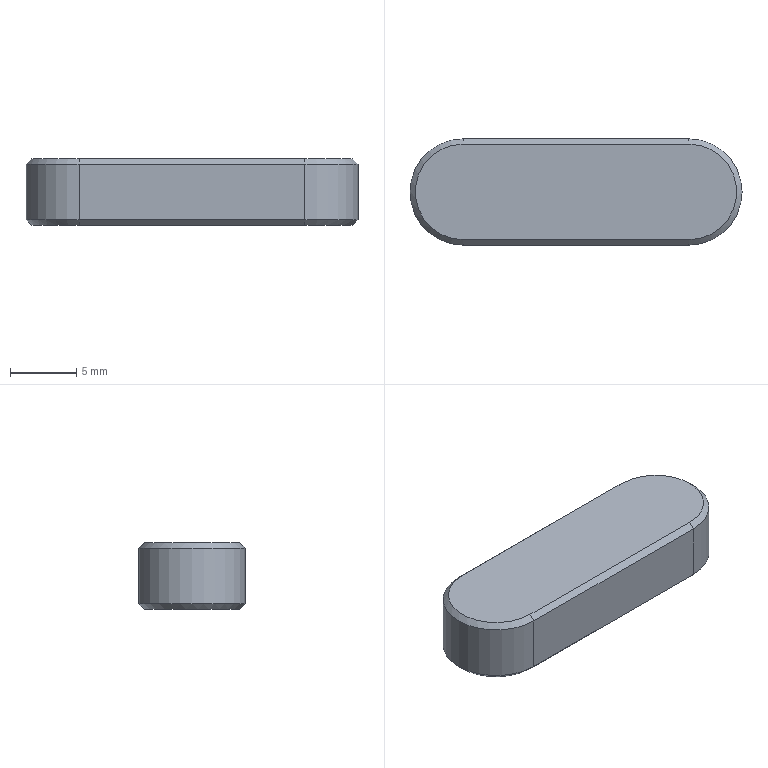Part | SolidWorks | features BaseBody 1 | 1 solid | 14 faces | box 25 x 8 x 5 mm | volume 922 mm3 | plane 8 | cone 4 | cylinder 2 | commonest cylinder face diameters 8 x2
STEP:
#1=CARTESIAN_POINT('',(21.,-3.6,-3.));
#2=VERTEX_POINT('',#1);
#3=CARTESIAN_POINT('',(21.,-4.,-2.6));
#4=VERTEX_POINT('',#3);
#5=CARTESIAN_POINT('',(21.,-3.6,-3.));
#6=DIRECTION('',(0.,-0.7071,0.7071));
#7=VECTOR('',#6,1000.);
#8=LINE('',#5,#7);
#9=EDGE_CURVE('',#2,#4,#8,.T.);
#10=ORIENTED_EDGE('',*,*,#9,.T.);
#11=CARTESIAN_POINT('',(4.,-4.,-2.6));
#12=VERTEX_POINT('',#11);
#13=CARTESIAN_POINT('',(8.25,-4.,-2.6));
#14=DIRECTION('',(-1.,0.,0.));
#15=VECTOR('',#14,1000.);
#16=LINE('',#13,#15);
#17=EDGE_CURVE('',#4,#12,#16,.T.);
#18=ORIENTED_EDGE('',*,*,#17,.T.);
#19=CARTESIAN_POINT('',(4.,-3.6,-3.));
#20=VERTEX_POINT('',#19);
#21=CARTESIAN_POINT('',(4.,-4.,-2.6));
#22=DIRECTION('',(0.,0.7071,-0.7071));
#23=VECTOR('',#22,1000.);
#24=LINE('',#21,#23);
#25=EDGE_CURVE('',#12,#20,#24,.T.);
#26=ORIENTED_EDGE('',*,*,#25,.T.);
#27=CARTESIAN_POINT('',(8.25,-3.6,-3.));
#28=DIRECTION('',(1.,0.,0.));
#29=VECTOR('',#28,1000.);
#30=LINE('',#27,#29);
#31=EDGE_CURVE('',#20,#2,#30,.T.);
#32=ORIENTED_EDGE('',*,*,#31,.T.);
#33=EDGE_LOOP('',(#10,#18,#26,#32));
#34=FACE_OUTER_BOUND('',#33,.T.);
#35=CARTESIAN_POINT('',(8.25,-3.8,-2.8));
#36=DIRECTION('',(0.,-0.7071,-0.7071));
#37=DIRECTION('',(0.,0.7071,-0.7071));
#38=AXIS2_PLACEMENT_3D('',#35,#36,#37);
#39=PLANE('',#38);
#40=ADVANCED_FACE('',(#34),#39,.T.);
#41=CARTESIAN_POINT('',(21.,3.6,-3.));
#42=VERTEX_POINT('',#41);
#43=CARTESIAN_POINT('',(21.,4.,-2.6));
#44=VERTEX_POINT('',#43);
#45=CARTESIAN_POINT('',(21.,3.6,-3.));
#46=DIRECTION('',(0.,0.7071,0.7071));
#47=VECTOR('',#46,1000.);
#48=LINE('',#45,#47);
#49=EDGE_CURVE('',#42,#44,#48,.T.);
#50=ORIENTED_EDGE('',*,*,#49,.T.);
#51=CARTESIAN_POINT('',(21.,0.,-2.6));
#52=DIRECTION('',(0.,0.,-1.));
#53=DIRECTION('',(0.,1.,0.));
#54=AXIS2_PLACEMENT_3D('',#51,#52,#53);
#55=CIRCLE('',#54,4.);
#56=EDGE_CURVE('',#44,#4,#55,.T.);
#57=ORIENTED_EDGE('',*,*,#56,.T.);
#58=ORIENTED_EDGE('',*,*,#9,.F.);
#59=CARTESIAN_POINT('',(21.,0.,-3.));
#60=DIRECTION('',(0.,0.,1.));
#61=DIRECTION('',(0.,1.,0.));
#62=AXIS2_PLACEMENT_3D('',#59,#60,#61);
#63=CIRCLE('',#62,3.6);
#64=EDGE_CURVE('',#2,#42,#63,.T.);
#65=ORIENTED_EDGE('',*,*,#64,.T.);
#66=EDGE_LOOP('',(#50,#57,#58,#65));
#67=FACE_OUTER_BOUND('',#66,.T.);
#68=CARTESIAN_POINT('',(21.,0.,-2.8));
#69=DIRECTION('',(0.,0.,1.));
#70=DIRECTION('',(0.,1.,0.));
#71=AXIS2_PLACEMENT_3D('',#68,#69,#70);
#72=CONICAL_SURFACE('',#71,3.8,0.7854);
#73=ADVANCED_FACE('',(#67),#72,.T.);
#74=CARTESIAN_POINT('',(4.,4.,-2.6));
#75=VERTEX_POINT('',#74);
#76=CARTESIAN_POINT('',(4.,3.6,-3.));
#77=VERTEX_POINT('',#76);
#78=CARTESIAN_POINT('',(4.,4.,-2.6));
#79=DIRECTION('',(0.,-0.7071,-0.7071));
#80=VECTOR('',#79,1000.);
#81=LINE('',#78,#80);
#82=EDGE_CURVE('',#75,#77,#81,.T.);
#83=ORIENTED_EDGE('',*,*,#82,.T.);
#84=CARTESIAN_POINT('',(4.,0.,-3.));
#85=DIRECTION('',(0.,0.,1.));
#86=DIRECTION('',(0.,-1.,0.));
#87=AXIS2_PLACEMENT_3D('',#84,#85,#86);
#88=CIRCLE('',#87,3.6);
#89=EDGE_CURVE('',#77,#20,#88,.T.);
#90=ORIENTED_EDGE('',*,*,#89,.T.);
#91=ORIENTED_EDGE('',*,*,#25,.F.);
#92=CARTESIAN_POINT('',(4.,0.,-2.6));
#93=DIRECTION('',(0.,0.,-1.));
#94=DIRECTION('',(0.,-1.,0.));
#95=AXIS2_PLACEMENT_3D('',#92,#93,#94);
#96=CIRCLE('',#95,4.);
#97=EDGE_CURVE('',#12,#75,#96,.T.);
#98=ORIENTED_EDGE('',*,*,#97,.T.);
#99=EDGE_LOOP('',(#83,#90,#91,#98));
#100=FACE_OUTER_BOUND('',#99,.T.);
#101=CARTESIAN_POINT('',(4.,0.,-2.8));
#102=DIRECTION('',(0.,0.,1.));
#103=DIRECTION('',(0.,-1.,0.));
#104=AXIS2_PLACEMENT_3D('',#101,#102,#103);
#105=CONICAL_SURFACE('',#104,3.8,0.7854);
#106=ADVANCED_FACE('',(#100),#105,.T.);
#107=ORIENTED_EDGE('',*,*,#49,.F.);
#108=CARTESIAN_POINT('',(16.75,3.6,-3.));
#109=DIRECTION('',(-1.,0.,0.));
#110=VECTOR('',#109,1000.);
#111=LINE('',#108,#110);
#112=EDGE_CURVE('',#42,#77,#111,.T.);
#113=ORIENTED_EDGE('',*,*,#112,.T.);
#114=ORIENTED_EDGE('',*,*,#82,.F.);
#115=CARTESIAN_POINT('',(16.75,4.,-2.6));
#116=DIRECTION('',(1.,0.,0.));
#117=VECTOR('',#116,1000.);
#118=LINE('',#115,#117);
#119=EDGE_CURVE('',#75,#44,#118,.T.);
#120=ORIENTED_EDGE('',*,*,#119,.T.);
#121=EDGE_LOOP('',(#107,#113,#114,#120));
#122=FACE_OUTER_BOUND('',#121,.T.);
#123=CARTESIAN_POINT('',(16.75,3.8,-2.8));
#124=DIRECTION('',(0.,0.7071,-0.7071));
#125=DIRECTION('',(-1.,0.,0.));
#126=AXIS2_PLACEMENT_3D('',#123,#124,#125);
#127=PLANE('',#126);
#128=ADVANCED_FACE('',(#122),#127,.T.);
#129=ORIENTED_EDGE('',*,*,#97,.F.);
#130=CARTESIAN_POINT('',(4.,-4.,1.6));
#131=VERTEX_POINT('',#130);
#132=CARTESIAN_POINT('',(4.,-4.,0.));
#133=DIRECTION('',(0.,0.,-1.));
#134=VECTOR('',#133,1000.);
#135=LINE('',#132,#134);
#136=EDGE_CURVE('',#131,#12,#135,.T.);
#137=ORIENTED_EDGE('',*,*,#136,.F.);
#138=CARTESIAN_POINT('',(4.,4.,1.6));
#139=VERTEX_POINT('',#138);
#140=CARTESIAN_POINT('',(4.,0.,1.6));
#141=DIRECTION('',(0.,0.,1.));
#142=DIRECTION('',(0.,-1.,0.));
#143=AXIS2_PLACEMENT_3D('',#140,#141,#142);
#144=CIRCLE('',#143,4.);
#145=EDGE_CURVE('',#139,#131,#144,.T.);
#146=ORIENTED_EDGE('',*,*,#145,.F.);
#147=CARTESIAN_POINT('',(4.,4.,0.));
#148=DIRECTION('',(0.,0.,1.));
#149=VECTOR('',#148,1000.);
#150=LINE('',#147,#149);
#151=EDGE_CURVE('',#75,#139,#150,.T.);
#152=ORIENTED_EDGE('',*,*,#151,.F.);
#153=EDGE_LOOP('',(#129,#137,#146,#152));
#154=FACE_OUTER_BOUND('',#153,.T.);
#155=CARTESIAN_POINT('',(4.,0.,0.));
#156=DIRECTION('',(0.,0.,1.));
#157=DIRECTION('',(0.,-1.,0.));
#158=AXIS2_PLACEMENT_3D('',#155,#156,#157);
#159=CYLINDRICAL_SURFACE('',#158,4.);
#160=ADVANCED_FACE('',(#154),#159,.T.);
#161=ORIENTED_EDGE('',*,*,#17,.F.);
#162=CARTESIAN_POINT('',(21.,-4.,1.6));
#163=VERTEX_POINT('',#162);
#164=CARTESIAN_POINT('',(21.,-4.,0.));
#165=DIRECTION('',(0.,0.,-1.));
#166=VECTOR('',#165,1000.);
#167=LINE('',#164,#166);
#168=EDGE_CURVE('',#163,#4,#167,.T.);
#169=ORIENTED_EDGE('',*,*,#168,.F.);
#170=CARTESIAN_POINT('',(8.25,-4.,1.6));
#171=DIRECTION('',(1.,0.,0.));
#172=VECTOR('',#171,1000.);
#173=LINE('',#170,#172);
#174=EDGE_CURVE('',#131,#163,#173,.T.);
#175=ORIENTED_EDGE('',*,*,#174,.F.);
#176=ORIENTED_EDGE('',*,*,#136,.T.);
#177=EDGE_LOOP('',(#161,#169,#175,#176));
#178=FACE_OUTER_BOUND('',#177,.T.);
#179=CARTESIAN_POINT('',(4.,-4.,0.));
#180=DIRECTION('',(0.,-1.,0.));
#181=DIRECTION('',(0.,0.,-1.));
#182=AXIS2_PLACEMENT_3D('',#179,#180,#181);
#183=PLANE('',#182);
#184=ADVANCED_FACE('',(#178),#183,.T.);
#185=ORIENTED_EDGE('',*,*,#31,.F.);
#186=ORIENTED_EDGE('',*,*,#89,.F.);
#187=ORIENTED_EDGE('',*,*,#112,.F.);
#188=ORIENTED_EDGE('',*,*,#64,.F.);
#189=EDGE_LOOP('',(#185,#186,#187,#188));
#190=FACE_OUTER_BOUND('',#189,.T.);
#191=CARTESIAN_POINT('',(12.5,0.,-3.));
#192=DIRECTION('',(0.,0.,1.));
#193=DIRECTION('',(1.,0.,0.));
#194=AXIS2_PLACEMENT_3D('',#191,#192,#193);
#195=PLANE('',#194);
#196=ADVANCED_FACE('',(#190),#195,.F.);
#197=CARTESIAN_POINT('',(4.,-3.6,2.));
#198=VERTEX_POINT('',#197);
#199=CARTESIAN_POINT('',(4.,-4.,1.6));
#200=DIRECTION('',(0.,0.7071,0.7071));
#201=VECTOR('',#200,1000.);
#202=LINE('',#199,#201);
#203=EDGE_CURVE('',#131,#198,#202,.T.);
#204=ORIENTED_EDGE('',*,*,#203,.T.);
#205=CARTESIAN_POINT('',(4.,3.6,2.));
#206=VERTEX_POINT('',#205);
#207=CARTESIAN_POINT('',(4.,0.,2.));
#208=DIRECTION('',(0.,0.,-1.));
#209=DIRECTION('',(0.,-1.,0.));
#210=AXIS2_PLACEMENT_3D('',#207,#208,#209);
#211=CIRCLE('',#210,3.6);
#212=EDGE_CURVE('',#198,#206,#211,.T.);
#213=ORIENTED_EDGE('',*,*,#212,.T.);
#214=CARTESIAN_POINT('',(4.,3.6,2.));
#215=DIRECTION('',(0.,0.7071,-0.7071));
#216=VECTOR('',#215,1000.);
#217=LINE('',#214,#216);
#218=EDGE_CURVE('',#206,#139,#217,.T.);
#219=ORIENTED_EDGE('',*,*,#218,.T.);
#220=ORIENTED_EDGE('',*,*,#145,.T.);
#221=EDGE_LOOP('',(#204,#213,#219,#220));
#222=FACE_OUTER_BOUND('',#221,.T.);
#223=CARTESIAN_POINT('',(4.,0.,1.8));
#224=DIRECTION('',(0.,0.,-1.));
#225=DIRECTION('',(0.,-1.,0.));
#226=AXIS2_PLACEMENT_3D('',#223,#224,#225);
#227=CONICAL_SURFACE('',#226,3.8,0.7854);
#228=ADVANCED_FACE('',(#222),#227,.T.);
#229=CARTESIAN_POINT('',(21.,-3.6,2.));
#230=VERTEX_POINT('',#229);
#231=CARTESIAN_POINT('',(21.,-4.,1.6));
#232=DIRECTION('',(0.,0.7071,0.7071));
#233=VECTOR('',#232,1000.);
#234=LINE('',#231,#233);
#235=EDGE_CURVE('',#163,#230,#234,.T.);
#236=ORIENTED_EDGE('',*,*,#235,.T.);
#237=CARTESIAN_POINT('',(8.25,-3.6,2.));
#238=DIRECTION('',(-1.,0.,0.));
#239=VECTOR('',#238,1000.);
#240=LINE('',#237,#239);
#241=EDGE_CURVE('',#230,#198,#240,.T.);
#242=ORIENTED_EDGE('',*,*,#241,.T.);
#243=ORIENTED_EDGE('',*,*,#203,.F.);
#244=ORIENTED_EDGE('',*,*,#174,.T.);
#245=EDGE_LOOP('',(#236,#242,#243,#244));
#246=FACE_OUTER_BOUND('',#245,.T.);
#247=CARTESIAN_POINT('',(8.25,-3.8,1.8));
#248=DIRECTION('',(0.,-0.7071,0.7071));
#249=DIRECTION('',(-1.,0.,0.));
#250=AXIS2_PLACEMENT_3D('',#247,#248,#249);
#251=PLANE('',#250);
#252=ADVANCED_FACE('',(#246),#251,.T.);
#253=CARTESIAN_POINT('',(21.,3.6,2.));
#254=VERTEX_POINT('',#253);
#255=CARTESIAN_POINT('',(21.,4.,1.6));
#256=VERTEX_POINT('',#255);
#257=CARTESIAN_POINT('',(21.,3.6,2.));
#258=DIRECTION('',(0.,0.7071,-0.7071));
#259=VECTOR('',#258,1000.);
#260=LINE('',#257,#259);
#261=EDGE_CURVE('',#254,#256,#260,.T.);
#262=ORIENTED_EDGE('',*,*,#261,.T.);
#263=CARTESIAN_POINT('',(16.75,4.,1.6));
#264=DIRECTION('',(-1.,0.,0.));
#265=VECTOR('',#264,1000.);
#266=LINE('',#263,#265);
#267=EDGE_CURVE('',#256,#139,#266,.T.);
#268=ORIENTED_EDGE('',*,*,#267,.T.);
#269=ORIENTED_EDGE('',*,*,#218,.F.);
#270=CARTESIAN_POINT('',(16.75,3.6,2.));
#271=DIRECTION('',(1.,0.,0.));
#272=VECTOR('',#271,1000.);
#273=LINE('',#270,#272);
#274=EDGE_CURVE('',#206,#254,#273,.T.);
#275=ORIENTED_EDGE('',*,*,#274,.T.);
#276=EDGE_LOOP('',(#262,#268,#269,#275));
#277=FACE_OUTER_BOUND('',#276,.T.);
#278=CARTESIAN_POINT('',(16.75,3.8,1.8));
#279=DIRECTION('',(0.,0.7071,0.7071));
#280=DIRECTION('',(1.,0.,0.));
#281=AXIS2_PLACEMENT_3D('',#278,#279,#280);
#282=PLANE('',#281);
#283=ADVANCED_FACE('',(#277),#282,.T.);
#284=ORIENTED_EDGE('',*,*,#235,.F.);
#285=CARTESIAN_POINT('',(21.,0.,1.6));
#286=DIRECTION('',(0.,0.,1.));
#287=DIRECTION('',(0.,1.,0.));
#288=AXIS2_PLACEMENT_3D('',#285,#286,#287);
#289=CIRCLE('',#288,4.);
#290=EDGE_CURVE('',#163,#256,#289,.T.);
#291=ORIENTED_EDGE('',*,*,#290,.T.);
#292=ORIENTED_EDGE('',*,*,#261,.F.);
#293=CARTESIAN_POINT('',(21.,0.,2.));
#294=DIRECTION('',(0.,0.,-1.));
#295=DIRECTION('',(0.,1.,0.));
#296=AXIS2_PLACEMENT_3D('',#293,#294,#295);
#297=CIRCLE('',#296,3.6);
#298=EDGE_CURVE('',#254,#230,#297,.T.);
#299=ORIENTED_EDGE('',*,*,#298,.T.);
#300=EDGE_LOOP('',(#284,#291,#292,#299));
#301=FACE_OUTER_BOUND('',#300,.T.);
#302=CARTESIAN_POINT('',(21.,0.,1.8));
#303=DIRECTION('',(0.,0.,-1.));
#304=DIRECTION('',(0.,1.,0.));
#305=AXIS2_PLACEMENT_3D('',#302,#303,#304);
#306=CONICAL_SURFACE('',#305,3.8,0.7854);
#307=ADVANCED_FACE('',(#301),#306,.T.);
#308=ORIENTED_EDGE('',*,*,#212,.F.);
#309=ORIENTED_EDGE('',*,*,#241,.F.);
#310=ORIENTED_EDGE('',*,*,#298,.F.);
#311=ORIENTED_EDGE('',*,*,#274,.F.);
#312=EDGE_LOOP('',(#308,#309,#310,#311));
#313=FACE_OUTER_BOUND('',#312,.T.);
#314=CARTESIAN_POINT('',(12.5,0.,2.));
#315=DIRECTION('',(0.,0.,1.));
#316=DIRECTION('',(1.,0.,0.));
#317=AXIS2_PLACEMENT_3D('',#314,#315,#316);
#318=PLANE('',#317);
#319=ADVANCED_FACE('',(#313),#318,.T.);
#320=ORIENTED_EDGE('',*,*,#119,.F.);
#321=ORIENTED_EDGE('',*,*,#151,.T.);
#322=ORIENTED_EDGE('',*,*,#267,.F.);
#323=CARTESIAN_POINT('',(21.,4.,0.));
#324=DIRECTION('',(0.,0.,-1.));
#325=VECTOR('',#324,1000.);
#326=LINE('',#323,#325);
#327=EDGE_CURVE('',#256,#44,#326,.T.);
#328=ORIENTED_EDGE('',*,*,#327,.T.);
#329=EDGE_LOOP('',(#320,#321,#322,#328));
#330=FACE_OUTER_BOUND('',#329,.T.);
#331=CARTESIAN_POINT('',(21.,4.,0.));
#332=DIRECTION('',(0.,1.,0.));
#333=DIRECTION('',(1.,0.,0.));
#334=AXIS2_PLACEMENT_3D('',#331,#332,#333);
#335=PLANE('',#334);
#336=ADVANCED_FACE('',(#330),#335,.T.);
#337=ORIENTED_EDGE('',*,*,#56,.F.);
#338=ORIENTED_EDGE('',*,*,#327,.F.);
#339=ORIENTED_EDGE('',*,*,#290,.F.);
#340=ORIENTED_EDGE('',*,*,#168,.T.);
#341=EDGE_LOOP('',(#337,#338,#339,#340));
#342=FACE_OUTER_BOUND('',#341,.T.);
#343=CARTESIAN_POINT('',(21.,0.,0.));
#344=DIRECTION('',(0.,0.,1.));
#345=DIRECTION('',(0.,1.,0.));
#346=AXIS2_PLACEMENT_3D('',#343,#344,#345);
#347=CYLINDRICAL_SURFACE('',#346,4.);
#348=ADVANCED_FACE('',(#342),#347,.T.);
#349=CLOSED_SHELL('',(#40,#73,#106,#128,#160,#184,#196,#228,#252,#283,#307,#319,#336,#348));
#350=MANIFOLD_SOLID_BREP('',#349);
#351=CARTESIAN_POINT('',(0.,0.,0.));
#352=DIRECTION('',(0.,0.,1.));
#353=DIRECTION('',(1.,0.,0.));
#354=AXIS2_PLACEMENT_3D('',#351,#352,#353);
#355=(LENGTH_UNIT()NAMED_UNIT(*)SI_UNIT(.MILLI.,.METRE.));
#356=UNCERTAINTY_MEASURE_WITH_UNIT(LENGTH_MEASURE(0.00001),#355,'','');
#357=(NAMED_UNIT(*)PLANE_ANGLE_UNIT()SI_UNIT($,.RADIAN.));
#358=(NAMED_UNIT(*)SI_UNIT($,.STERADIAN.)SOLID_ANGLE_UNIT());
#359=(GEOMETRIC_REPRESENTATION_CONTEXT(3)GLOBAL_UNCERTAINTY_ASSIGNED_CONTEXT((#356))GLOBAL_UNIT_ASSIGNED_CONTEXT((#355,#357,#358))REPRESENTATION_CONTEXT('',''));
#360=ADVANCED_BREP_SHAPE_REPRESENTATION('',(#350,#354),#359);